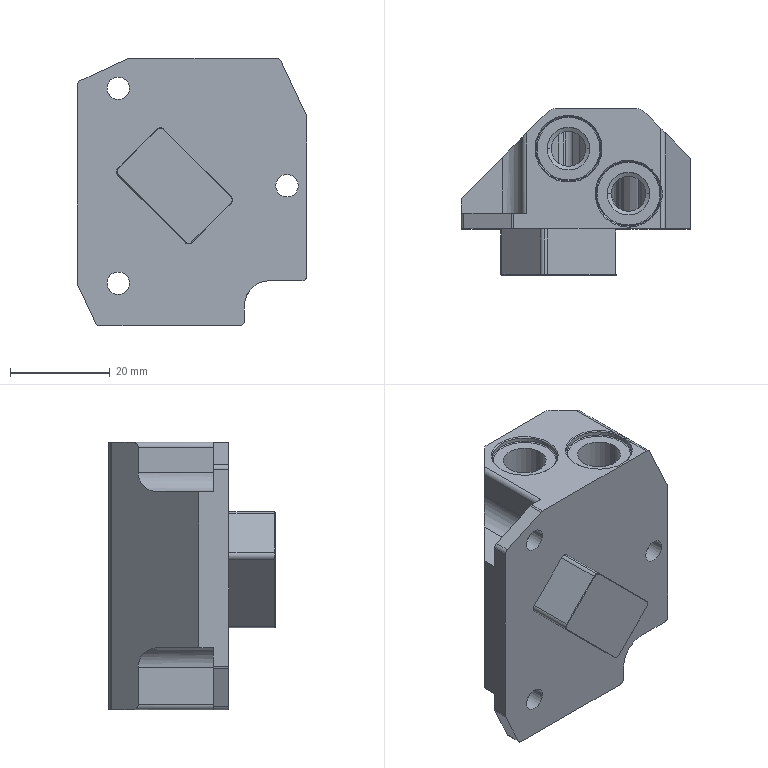NC program | NX | posted with a generic post | part box 46 x 33.25 x 53.5 mm
Lines 19 to 841 of 9227:
(动态粗 , TOOL : D10-30-D10-75-3T-ROUGH)
N36 T02 M6
N38 G53
N40 G17 G0 G90 X35.793 Y-2.826 B0. C0. S5500 M3
N42 G43 Z30.2 H2
N44 Z-24.5
N46 G94 G1 X35.768 Y-2.825 Z-24.656 F1500.
N48 X35.743 Y-2.824 Z-24.718
N50 X35.718 Y-2.823 Z-24.763
N52 X35.693 Y-2.822 Z-24.8
N54 X35.668 Y-2.821 Z-24.831
N56 X35.643 Y-2.82 Z-24.857
N58 X35.618 Y-2.819 Z-24.88
N60 X35.593 Y-2.818 Z-24.9
N62 X35.568 Y-2.817 Z-24.918
N64 X35.543 Y-2.816 Z-24.933
N66 X35.518 Y-2.815 Z-24.947
N68 X35.493 Y-2.814 Z-24.958
N70 X35.468 Y-2.813 Z-24.968
N72 X35.443 Y-2.812 Z-24.977
N74 X35.418 Y-2.811 Z-24.984
N76 X35.393 Y-2.81 Z-24.99
N78 X35.368 Y-2.809 Z-24.994
N80 X35.343 Y-2.808 Z-24.997
N82 X35.318 Y-2.807 Z-24.999
N84 X35.293 Y-2.806 Z-25.
N86 X33.787 Y-2.747
N88 G3 X32.775 Y-3.481 R1.01
N90 X32.348 Y-6.702 R13.384
N92 G1 X32.245 Y-11.061
N94 G2 X31.896 Y-13.227 R14.737
N96 X31.329 Y-15.21 R7.148
N98 X27.785 Y-23.176 R150.474
N100 X26.718 Y-25.28 R15.121
N102 X22.414 Y-28.199 R7.784
N104 X17.525 Y-28.893 R20.84
N106 X6.201 Y-28.999 R306.779
N108 G1 X-16.874 Y-28.998
N110 G2 X-21.685 Y-27.937 R14.794
N112 X-28.661 Y-24.862 R88.391
N114 X-31.659 Y-21.135 R7.243
N116 X-32.586 Y-16.368 R16.374
N118 X-32.747 Y-7.596 R145.919
N120 G1 X-32.75 Y-3.096
N122 G2 X-32.733 Y10.261 R991.956
N124 X-30.343 Y14.303 R5.749
N126 X-26.662 Y15.925 R9.882
N128 G3 X-24.702 Y16.523 R9.347
N130 X-24.139 Y17.376 R1.119
N132 X-23.808 Y21.173 R21.778
N134 G2 X-23.699 Y23.253 R13.999
N136 X-20.868 Y27.145 R6.06
N138 X-16.339 Y28.654 R11.322
N140 X-10.239 Y28.977 R49.941
N142 G1 X-1.314 Y29.
N144 X13.211 Y28.998
N146 G2 X17.775 Y28.028 R14.405
N148 X24.908 Y24.933 R98.139
N150 X28.234 Y23.354 R61.251
N152 X30.841 Y20.415 R7.126
N154 G1 X30.98 Y20.237
N156 X31.512 Y19.195
N158 G2 X32.063 Y16.21 R10.538
N160 X32.246 Y7.889 R121.537
N162 G1 X32.25 Y2.714
N164 G2 X32.234 Y-9.235 R902.524
N166 G3 X31.95 Y-10.575 R62.037
N168 G2 X31.884 Y-13.384 R26.459
N170 X31.369 Y-15.105 R6.543
N172 G1 X26.932 Y-24.621
N174 X26.338 Y-25.631
N176 X25.567 Y-26.511
N178 X24.643 Y-27.23
N180 X23.601 Y-27.762
N182 X22.477 Y-28.09
N184 G2 X16.086 Y-28.423 R88.323
N186 X3.336 Y-28.499 R660.995
N188 G1 X-15.051 Y-28.498
N190 G2 X-18.406 Y-28.176 R18.904
N192 X-20.71 Y-27.663 R7.341
N194 X-26.906 Y-25.084 R50.581
N196 X-28.468 Y-23.983 R10.692
N198 G1 X-29.381 Y-23.446
N200 X-30.261 Y-22.674
N202 X-30.98 Y-21.751
N204 X-31.512 Y-20.709
N206 X-31.84 Y-19.585
N208 G2 X-32.225 Y-10.708 R96.838
N210 G1 X-32.249 Y-1.108
N212 G2 X-32.232 Y8.223 R534.374
N214 X-31.934 Y9.881 R9.532
N216 X-26.362 Y15.669 R6.203
N218 G3 X-24.57 Y16.389 R3.889
N220 X-23.862 Y17.732 R2.705
N222 X-23.399 Y20.922 R18.234
N224 G2 X-22.838 Y23.021 R9.161
N226 G1 X-22.762 Y23.515
N228 X-22.37 Y24.619
N230 X-21.777 Y25.629
N232 X-21.005 Y26.509
N234 X-20.081 Y27.229
N236 X-19.039 Y27.762
N238 X-17.914 Y28.09
N240 G2 X-8.605 Y28.478 R100.527
N242 G1 X-0.355 Y28.499
N244 G2 X12.086 Y28.483 R926.244
N246 X14.656 Y28.2 R21.713
N248 X17.449 Y27.619 R6.654
N250 X26.375 Y23.663 R119.47
N252 X27.507 Y22.929 R30.959
N254 X29.381 Y21.933 R12.327
N256 G1 X30.261 Y21.161
N258 X30.86 Y20.391
N260 X30.261 Y21.161
N262 X29.381 Y21.933
N264 G3 X27.507 Y22.929 R12.327
N266 G1 X17.449 Y27.619
N268 G3 X14.656 Y28.2 R6.624
N270 G1 X-16.749
N272 X-17.914 Y28.09
N274 X-19.039 Y27.762
N276 X-20.081 Y27.229
N278 X-21.005 Y26.509
N280 X-21.777 Y25.629
N282 X-22.37 Y24.619
N284 X-22.762 Y23.515
N286 G3 X-23.224 Y19.783 R77.333
N288 G2 X-23.913 Y17.107 R8.828
N290 X-25.837 Y15.697 R2.696
N292 G3 X-26.589 Y15.628 R10.459
N294 G2 X-25.425 Y15.727 R25.281
N296 G3 X-23.638 Y17.249 R2.66
N298 X-22.95 Y19.454 R8.395
N300 G1 X-22.94 Y22.357
N302 G2 X-22.972 Y18.942 R91.453
N304 X-24.268 Y16.215 R4.314
N306 X-25.661 Y15.697 R1.792
N308 G3 X-23.723 Y16.556 R2.139
N310 X-22.95 Y18.084 R3.195
N312 G1 Y19.247
N314 G2 X-22.971 Y17.827 R14.78
N316 X-24.704 Y15.732 R2.841
N318 X-25.143 Y15.699 R6.429
N320 G3 X-23.597 Y16.317 R1.818
N322 X-22.95 Y17.469 R1.983
N324 G1 Y18.032
N326 G2 X-22.983 Y17.179 R3.888
N328 X-24.412 Y15.717 R2.152
N330 G1 X-24.786 Y15.7
N332 G3 X-23.244 Y16.394 R1.668
N334 X-22.95 Y17.418 R1.288
N336 G2 X-23.709 Y15.879 R1.538
N338 X-24.426 Y15.7 R1.168
N340 G3 X-22.95 Y17.059 R1.284
N342 G2 X-24.162 Y15.7 R1.183
N344 G3 X-22.959 Y16.708 R1.089
N346 G2 X-23.845 Y15.72 R1.054
N348 X-26.143 Y15.688 R53.417
N350 G3 X-31.95 Y9.5 R6.211
N352 G1 Y-18.42
N354 X-31.84 Y-19.585
N356 X-31.512 Y-20.709
N358 X-30.98 Y-21.751
N360 X-30.261 Y-22.674
N362 X-29.381 Y-23.446
N364 G3 X-26.506 Y-24.94 R24.613
N366 X-23.307 Y-26.404 R59.619
N368 G1 X-20.695 Y-27.619
N370 X-19.854 Y-27.939
N372 X-20.695 Y-27.619
N374 X-28.234 Y-24.103
N376 X-20.695 Y-27.619
N378 G3 X-18.075 Y-28.2 R6.608
N380 G1 X21.312
N382 G2 X21.972 Y-28.448 R1.005
N384 G1 X22.508 Y-28.919
N386 X23.998 Y-30.226 Z-24.9
N388 G3 X25.175 Y-30.43 R1.026 F15000.
N390 G1 X25.866 Y-30.088
N392 X26.549 Y-29.732
N394 G3 X28.082 Y-28.293 R4.702
N396 X30.353 Y-24.623 R45.308
N398 X32.163 Y-21.176 R57.483
N400 X33.537 Y-17.922 R42.581
N402 G1 X35.104 Y-13.729
N404 G3 X34.6 Y-12.477 R1.
N406 G1 X34.441 Y-12.401
N408 X32.654 Y-11.542 Z-25. F1500.
N410 G2 X32.103 Y-11.107 R1.163
N412 X31.95 Y-10.575 R1.013
N414 G1 Y16.907
N416 X31.84 Y18.071
N418 G2 X32.444 Y19.093 R1.01
N420 G1 X33.935 Y19.738
N422 X33.958 Y19.748 Z-24.999
N424 X33.981 Y19.758 Z-24.997
N426 X34.004 Y19.768 Z-24.994
N428 X34.027 Y19.778 Z-24.99
N430 X34.05 Y19.788 Z-24.984
N432 X34.073 Y19.797 Z-24.977
N434 X34.096 Y19.807 Z-24.968
N436 X34.119 Y19.817 Z-24.958
N438 X34.142 Y19.827 Z-24.947
N440 X34.165 Y19.837 Z-24.933
N442 X34.187 Y19.847 Z-24.918
N444 X34.21 Y19.857 Z-24.9
N446 X34.233 Y19.867 Z-24.88
N448 X34.256 Y19.877 Z-24.857
N450 X34.279 Y19.887 Z-24.831
N452 X34.302 Y19.897 Z-24.8
N454 X34.325 Y19.907 Z-24.763
N456 X34.348 Y19.917 Z-24.718
N458 X34.371 Y19.926 Z-24.656
N460 X34.394 Y19.936 Z-24.5
N462 G0 Z30.2
N464 X34.919 Y-8.983
N466 Z-20.25
N468 G1 X34.894 Y-8.988 Z-20.406
N470 X34.87 Y-8.992 Z-20.468
N472 X34.845 Y-8.997 Z-20.513
N474 X34.821 Y-9.002 Z-20.55
N476 X34.796 Y-9.007 Z-20.581
N478 X34.772 Y-9.011 Z-20.607
N480 X34.747 Y-9.016 Z-20.63
N482 X34.723 Y-9.021 Z-20.65
N484 X34.698 Y-9.025 Z-20.668
N486 X34.673 Y-9.03 Z-20.683
N488 X34.649 Y-9.035 Z-20.697
N490 X34.624 Y-9.039 Z-20.708
N492 X34.6 Y-9.044 Z-20.718
N494 X34.575 Y-9.049 Z-20.727
N496 X34.551 Y-9.053 Z-20.734
N498 X34.526 Y-9.058 Z-20.74
N500 X34.502 Y-9.063 Z-20.744
N502 X34.477 Y-9.067 Z-20.747
N504 X34.452 Y-9.072 Z-20.749
N506 X34.428 Y-9.077 Z-20.75
N508 X32.722 Y-9.402
N510 G3 X31.906 Y-10.295 R1.01
N512 G2 X31.056 Y-14.012 R14.1
N514 X28.401 Y-20.262 R75.825
N516 X26.858 Y-23.475 R47.618
N518 X22.769 Y-26.709 R7.485
N520 X19.592 Y-27.417 R16.665
N522 G3 X18.824 Y-27.805 R19.475
N524 G1 X17.849 Y-28.1
N526 X17.214 Y-28.163
N528 G3 X19.551 Y-27.417 R4.892
N530 X22.182 Y-26.533 R101.684
N532 X26.36 Y-23.095 R8.995
N534 X28.937 Y-18.301 R32.428
N536 X30.941 Y-13.227 R41.328
N538 G1 X31.477 Y-12.224
N540 X31.83 Y-11.061
N542 X31.477 Y-12.224
N544 G2 X30.373 Y-14.168 R37.231
N546 G3 X27.811 Y-19.458 R525.404
N548 G2 X25.412 Y-23.188 R16.8
N550 X21.65 Y-25.856 R11.889
N552 G3 X20.769 Y-26.364 R2.983
N554 G2 X19.492 Y-27.448 R4.465
N556 G3 X20.841 Y-26.277 R4.557
N558 G2 X22.786 Y-24.915 R28.771
N560 G3 X26.923 Y-20.257 R14.47
N562 X29.554 Y-15.145 R84.07
N564 G2 X30.065 Y-14.292 R3.495
N566 X30.981 Y-14.073 R1.001
N568 X31.604 Y-14.549 Z-20.709 R1.062
N570 G1 X32.278 Y-15.516 Z-20.65
N572 X32.544 Y-15.905 F15000.
N574 X32.826 Y-16.283
N576 G3 X33.928 Y-16.522 R1.001
N578 X34.616 Y-15.84 R1.056
N580 X34.28 Y-14.769 R1.001
N582 G1 X33.347 Y-14.028
N584 X32.783 Y-13.576 Z-20.686 F1500.
N586 X32.212 Y-13.133 Z-20.723
N588 G3 X31.711 Y-12.961 Z-20.75 R1.005
N590 X30.88 Y-13.325 R1.002
N592 G2 X29.706 Y-14.636 R9.525
N594 G3 X28.14 Y-17.08 R16.696
N596 G2 X25.541 Y-21.266 R33.612
N598 X22.103 Y-24.604 R19.075
N600 G3 X21.565 Y-25.13 R2.381
N602 G2 X20.801 Y-26.325 R4.553
N604 G3 X21.565 Y-25.13 R4.553
N606 G2 X22.53 Y-24.018 R5.772
N608 G3 X27.3 Y-17.885 R25.805
N610 G2 X29.059 Y-15.12 R26.394
N612 G1 X29.17 Y-15.02
N614 G2 X30.131 Y-14.984 R1.001
N616 G1 X30.842 Y-15.439 Z-20.707
N618 X31.544 Y-15.906 Z-20.665
N620 X31.79 Y-16.068 Z-20.65
N622 X32.153 Y-16.303 F15000.
N624 X32.506 Y-16.552
N626 G2 X32.324 Y-18.173 R1.
N628 X31.88 Y-18.368 R1.466
N630 X30.801 Y-16.905 R1.
N632 G1 X31.481 Y-15.568 Z-20.726 F1500.
N634 G3 X31.561 Y-15.098 Z-20.75 R1.011
N636 X29.93 Y-14.401 R1.
N638 G1 X28.753 Y-15.336
N640 G3 X26.942 Y-17.681 R15.325
N642 G2 X22.471 Y-23.318 R39.283
N644 G3 X21.916 Y-24.078 R2.888
N646 G1 X21.604 Y-25.057
N648 X22.005 Y-23.847
N650 G2 X23.28 Y-22.075 R12.371
N652 G3 X27.053 Y-17.004 R85.206
N654 G2 X28.422 Y-15.421 R8.427
N656 G1 X29.115 Y-15.048
N658 G3 X27.629 Y-15.978 R6.454
N660 X25.208 Y-18.817 R24.169
N662 X22.369 Y-22.517 R82.134
N664 X22.008 Y-23.275 R2.038
N666 G1 X21.935 Y-24.016
N668 G2 X22.063 Y-22.987 R6.701
N670 X23.285 Y-20.905 R9.096
N672 X26.806 Y-16.471 R46.103
N674 X27.781 Y-15.682 R3.267
N676 G3 X28.254 Y-15.508 R2.699
N678 G2 X27.496 Y-15.78 R5.801
N680 G3 X25.578 Y-17.364 R7.119
N682 X22.344 Y-21.603 R25.212
N684 X22.036 Y-22.416 R1.987
N686 G1 X22.017 Y-23.187
N688 X22.038 Y-22.266
N690 G2 X22.97 Y-20.275 R5.838
N692 X26.279 Y-16.384 R18.594
N694 X26.95 Y-15.934 R3.562
N696 G1 X27.604 Y-15.735
N698 G3 X26.331 Y-16.183 R6.188
N700 X23.778 Y-18.524 R10.161
N702 X22.073 Y-21.226 R10.194
N704 X22.036 Y-22.347 R5.834
N706 G2 X22.058 Y-21.191 R10.596
N708 X23.243 Y-18.888 R6.735
N710 X26.005 Y-16.189 R9.856
N712 X26.958 Y-15.931 R1.713
N714 G3 X24.867 Y-16.739 R3.341
N716 X22.075 Y-20.277 R8.813
N718 X22.036 Y-21.409 R5.651
N720 G2 X22.058 Y-20.252 R10.443
N722 X23.441 Y-17.828 R6.024
N724 X25.691 Y-16.076 R6.255
N726 G1 X26.359 Y-15.99
N728 G3 X24.011 Y-16.909 R3.554
N730 X22.071 Y-19.442 R6.352
N732 X22.036 Y-20.451 R4.327
N734 G2 X22.089 Y-19.278 R4.722
N736 X25.128 Y-16.088 R5.398
N738 X25.749 Y-16.05 R2.961
N740 G3 X23.655 Y-16.728 R2.866
N742 X22.068 Y-18.726 R4.655
N744 X22.036 Y-19.618 R4.413
N746 G2 X22.065 Y-18.652 R5.206
N748 X24.653 Y-16.066 R4.087
N750 G1 X25.201 Y-16.05
N752 G3 X23.023 Y-16.825 R2.747
N754 X22.058 Y-18.173 R2.99
N756 X22.036 Y-18.9 R12.294
N758 G2 X22.068 Y-18.046 R3.962
N760 X24.165 Y-16.059 R3.109
N762 G1 X24.631 Y-16.05
N764 G3 X22.582 Y-16.859 R2.389
N766 X22.036 Y-18.268 R1.614
N768 G2 X22.192 Y-17.273 R1.791
N770 X23.708 Y-16.059 R2.402
N772 G1 X24.1 Y-16.05
N774 G3 X22.066 Y-17.296 R1.929
N776 X22.036 Y-17.831 R4.435
N778 G2 X22.719 Y-16.35 R1.512
N780 X23.672 Y-16.05 R1.32
N782 G3 X22.073 Y-16.998 R1.488
N784 X22.036 Y-17.482 R3.147
N786 G2 X23.309 Y-16.05 R1.25
N788 G3 X22.494 Y-16.246 R1.346
N790 X22.041 Y-17.096 R1.076
N792 G1 X22.036 Y-17.188
N794 G2 X22.221 Y-16.519 R1.243
N796 X22.754 Y-16.119 R1.034
N798 X23.993 Y-16.724 R1.01
N800 G1 X24.682 Y-18.528
N802 X24.69 Y-18.551 Z-20.749
N804 X24.699 Y-18.575 Z-20.747
N806 X24.708 Y-18.598 Z-20.744
N808 X24.717 Y-18.621 Z-20.74
N810 X24.726 Y-18.645 Z-20.734
N812 X24.735 Y-18.668 Z-20.727
N814 X24.744 Y-18.692 Z-20.718
N816 X24.753 Y-18.715 Z-20.708
N818 X24.762 Y-18.738 Z-20.697
N820 X24.771 Y-18.762 Z-20.683
N822 X24.78 Y-18.785 Z-20.668
N824 X24.789 Y-18.808 Z-20.65
N826 X24.798 Y-18.832 Z-20.63
N828 X24.806 Y-18.855 Z-20.607
N830 X24.815 Y-18.878 Z-20.581
N832 X24.824 Y-18.902 Z-20.55
N834 X24.833 Y-18.925 Z-20.513
N836 X24.842 Y-18.948 Z-20.468
N838 X24.851 Y-18.972 Z-20.406
N840 X24.86 Y-18.995 Z-20.25
N842 G0 Z30.2
N844 X-13.457 Y-31.172
N846 Z-20.25
N848 G1 X-13.461 Y-31.148 Z-20.406
N850 X-13.464 Y-31.123 Z-20.468
N852 X-13.468 Y-31.098 Z-20.513
N854 X-13.472 Y-31.073 Z-20.55
N856 X-13.475 Y-31.049 Z-20.581
N858 X-13.479 Y-31.024 Z-20.607
N860 X-13.483 Y-30.999 Z-20.63
N862 X-13.486 Y-30.975 Z-20.65
N864 X-13.49 Y-30.95 Z-20.668
N866 X-13.494 Y-30.925 Z-20.683
N868 X-13.498 Y-30.9 Z-20.697
N870 X-13.501 Y-30.876 Z-20.708
N872 X-13.505 Y-30.851 Z-20.718
N874 X-13.509 Y-30.826 Z-20.727
N876 X-13.512 Y-30.801 Z-20.734
N878 X-13.516 Y-30.777 Z-20.74
N880 X-13.52 Y-30.752 Z-20.744
N882 X-13.523 Y-30.727 Z-20.747
N884 X-13.527 Y-30.703 Z-20.749
N886 X-13.531 Y-30.678 Z-20.75
N888 X-13.778 Y-29.022
N890 G3 X-14.677 Y-28.166 R1.01
N892 G2 X-16.399 Y-27.916 R20.903
N894 X-21.244 Y-26.649 R17.69
N896 X-27.074 Y-24.047 R73.374
N898 X-30.423 Y-19.963 R7.43
N900 X-31.291 Y-15.297 R16.875
N902 G1 X-31.418 Y-12.413
N904 X-31.472 Y-12.234
N906 G3 X-32.02 Y-11.763 R1.004
N908 G1 X-32.461 Y-11.608
N910 X-34.33 Y-10.947 Z-20.65
N912 X-34.597 Y-10.851 F15000.
N914 X-34.868 Y-10.769
N916 G3 X-35.932 Y-12.234 R1.
N918 G1 X-35.815 Y-12.446
N920 X-35.689 Y-12.653
N922 G3 X-33.994 Y-12.489 R1.
N924 X-33.893 Y-11.949 Z-20.678 R1.135 F1500.
N926 G1 X-33.9 Y-10.522 Z-20.75
N928 G2 X-33.515 Y-9.61 R1.057
N930 X-31.906 Y-10.301 R1.
N932 G1 X-31.831 Y-11.058
N934 G2 X-31.325 Y-12.732 R28.885
N936 X-30.854 Y-16.508 R148.155
N938 G3 X-29.566 Y-20.596 R11.254
N940 X-26.196 Y-23.864 R9.827
N942 X-18.743 Y-27.088 R29.083
N944 G2 X-16.891 Y-27.505 R64.827
N946 G1 X-16.327 Y-27.803
N948 X-15.351 Y-28.1
N950 G2 X-17.226 Y-27.323 R6.073
N952 G3 X-21.161 Y-25.747 R202.118
N954 G2 X-25.892 Y-23.291 R24.946
N956 X-29.663 Y-17.993 R10.083
N958 X-30.581 Y-14. R33.2
N960 G3 X-30.906 Y-13.293 R1.294
N962 G1 X-31.471 Y-12.235
N964 X-30.906 Y-13.293
N966 G2 X-30.391 Y-14.328 R2.424
N968 G3 X-29.314 Y-17.877 R53.28
N970 X-24.691 Y-23.496 R11.223
N972 X-19.336 Y-26.124 R30.901
N974 G2 X-17.933 Y-26.742 R11.178
N976 G1 X-17.226 Y-27.323
N978 G3 X-20.119 Y-25.393 R11.781
N980 G2 X-24.276 Y-23.032 R33.212
N982 X-28.755 Y-17.218 R12.639
N984 G3 X-29.787 Y-14.594 R84.708
N986 G1 X-29.976 Y-14.363
N988 G3 X-30.845 Y-14.166 R1.002
N990 X-31.338 Y-14.446 Z-20.721 R1.101
N992 G1 X-32.398 Y-15.373 Z-20.65
N994 X-33.638 Y-16.457 F15000.
N996 G2 X-34.511 Y-16.73 R1.128
N998 X-34.865 Y-14.873 R1.
N1000 G1 X-33.357 Y-14.007
N1002 X-32.661 Y-13.604 Z-20.691 F1500.
N1004 X-31.96 Y-13.211 Z-20.731
N1006 X-31.785 Y-13.146 Z-20.741
N1008 X-31.602 Y-13.113 Z-20.75
N1010 G2 X-30.756 Y-13.476 R1.001
N1012 G1 X-30.135 Y-14.233
N1014 G2 X-29.419 Y-15.161 R2.282
N1016 G3 X-27.79 Y-18.449 R67.036
N1018 X-22.717 Y-23.541 R14.296
N1020 X-19.074 Y-25.645 R422.71
N1022 G2 X-18.535 Y-26.039 R5.066
N1024 G1 X-18.013 Y-26.676
N1026 G3 X-20.333 Y-24.527 R8.106
N1028 G2 X-24.016 Y-21.888 R35.914
N1030 X-27.715 Y-17.185 R16.834
N1032 G3 X-28.869 Y-15.239 R17.423
N1034 G1 X-29.071 Y-15.072
N1036 G3 X-30.052 Y-15.051 R1.001
N1038 G1 X-31.705 Y-16.145 Z-20.65
N1040 X-32.054 Y-16.374 F15000.
N1042 X-32.393 Y-16.616
N1044 G3 X-32.162 Y-18.262 R1.007
N1046 X-30.783 Y-16.92 R1.
N1048 G1 X-31.48 Y-15.574 Z-20.727 F1500.
N1050 G2 X-31.565 Y-15.12 Z-20.75 R1.013
N1052 X-29.932 Y-14.399 R1.
N1054 G3 X-28.851 Y-15.225 R10.073
N1056 G2 X-27.639 Y-16.861 R10.451
N1058 G3 X-23.913 Y-21.428 R20.905
N1060 X-20.195 Y-24.259 R45.953
N1062 G2 X-18.96 Y-25.331 R6.532
N1064 G1 X-18.66 Y-25.888
N1066 G3 X-20.266 Y-23.841 R5.548
N1068 G2 X-23.617 Y-20.924 R71.502
N1070 X-27.046 Y-16.757 R31.261
N1072 G3 X-28.004 Y-15.642 R5.431
N1074 G1 X-28.101 Y-15.585
N1076 G3 X-29.067 Y-15.758 R1.001
N1078 G1 X-30.547 Y-17.076 Z-20.65
N1080 X-31.303 Y-17.749 F15000.
N1082 G3 X-30.331 Y-19.448 R1.
N1084 X-29.716 Y-19.08 R1.161
N1086 X-29.599 Y-17.997 R1.001
N1088 G1 X-29.864 Y-17.473
N1090 X-30.42 Y-16.364 Z-20.713 F1500.
N1092 G2 X-30.445 Y-15.64 Z-20.75 R1.001
N1094 X-29.03 Y-15.093 R1.
N1096 X-27.781 Y-15.781 R12.344
N1098 X-26.211 Y-17.491 R13.038
N1100 G3 X-20.943 Y-22.853 R36.83
N1102 G2 X-19.303 Y-24.527 R10.316
N1104 G3 X-19.034 Y-25.187 R6.262
N1106 G2 X-19.332 Y-24.395 R4.429
N1108 G3 X-20.867 Y-22.456 R8.134
N1110 G2 X-26.06 Y-16.897 R88.533
N1112 G3 X-27.204 Y-15.865 R5.049
N1114 G1 X-28.124 Y-15.577
N1116 G2 X-27.048 Y-15.926 R14.317
N1118 X-25.149 Y-17.582 R9.073
N1120 G3 X-20.541 Y-22.401 R793.67
N1122 G2 X-19.49 Y-23.804 R6.457
N1124 G1 X-19.446 Y-23.948
N1126 G2 X-20.931 Y-24.994 R1.
N1128 X-21.356 Y-24.518 Z-20.717 R1.087
N1130 G1 X-21.987 Y-23.343 Z-20.65
N1132 G3 X-22.367 Y-22.856 R1.216 F15000.
N1134 X-23.906 Y-23.948 R1.
N1136 G1 X-23.808 Y-24.299
N1138 X-23.694 Y-24.646
N1140 G3 X-23.003 Y-25.204 R1.002
N1142 G1 X-21.595 Y-25.517
N1144 X-20.394 Y-25.779 Z-20.712 F1500.
N1146 G3 X-19.677 Y-25.616 Z-20.75 R1.001
N1148 X-19.287 Y-24.502 R1.
N1150 G1 X-19.546 Y-23.539
N1152 G3 X-21.065 Y-21.322 R8.951
N1154 X-25.29 Y-16.814 R65.506
N1156 X-26.398 Y-16.01 R3.98
N1158 G1 X-26.961 Y-15.93
N1160 X-27.212 Y-15.854
N1162 G3 X-26.425 Y-15.986 R2.968
N1164 G2 X-24.823 Y-17.012 R4.73
N1166 X-20.233 Y-21.97 R37.038
N1168 X-19.506 Y-23.315 R4.238
N1170 G1 X-19.447 Y-23.901
N1172 G3 X-20.251 Y-21.506 R4.202
N1174 X-24.76 Y-16.574 R22.329
N1176 X-25.751 Y-16.05 R2.362
N1178 G1 X-26.534 Y-15.973
N1180 G2 X-25.49 Y-16.093 R10.153
N1182 X-23.546 Y-17.359 R6.184
N1184 X-20.002 Y-21.511 R18.502
N1186 X-19.536 Y-22.653 R3.145
N1188 G1 X-19.521 Y-23.149
N1190 G3 X-19.59 Y-22.127 R6.741
N1192 X-20.941 Y-19.605 R7.555
N1194 X-24.181 Y-16.427 R13.415
N1196 X-25.074 Y-16.05 R2.04
N1198 G1 X-25.749
N1200 G2 X-24.68 Y-16.111 R3.709
N1202 X-22.471 Y-17.574 R6.507
N1204 X-19.734 Y-21.215 R11.626
N1206 X-19.536 Y-22.477 R2.427
N1208 G3 X-19.674 Y-20.986 R4.296
N1210 X-21.881 Y-17.662 R9.08
N1212 X-24.082 Y-16.085 R6.581
N1214 X-25.016 Y-16.05 R4.105
N1216 G2 X-24.01 Y-16.08 R5.105
N1218 X-21.903 Y-17.396 R5.411
N1220 X-19.573 Y-20.805 R8.403
N1222 X-19.536 Y-21.664 R3.636
N1224 G3 X-19.636 Y-20.256 R4.763
N1226 X-23.197 Y-16.129 R7.312
N1228 G1 X-23.549 Y-16.05
N1230 X-24.262
N1232 G2 X-23.256 Y-16.08 R5.107
N1234 X-21.134 Y-17.492 R5.002
N1236 X-19.545 Y-20.105 R6.146
N1238 G1 X-19.536 Y-20.806
N1240 G3 X-19.644 Y-19.423 R4.383
N1242 X-22.55 Y-16.109 R5.744
N1244 X-23.481 Y-16.05 R3.142
N1246 G2 X-22.443 Y-16.115 R3.432
N1248 X-20.068 Y-18.172 R4.947
N1250 X-19.536 Y-19.444 R3.169
N1252 G1 Y-20.006
N1254 G3 X-19.652 Y-18.672 R3.869
N1256 X-21.963 Y-16.097 R4.46
N1258 X-22.783 Y-16.05 R2.828
N1260 G2 X-21.79 Y-16.127 R2.762
N1262 X-19.542 Y-18.696 R3.913
N1264 G1 X-19.536 Y-19.221
N1266 G3 X-20.412 Y-16.833 R2.935
N1268 X-21.566 Y-16.064 R2.389
N1270 G1 X-22.176 Y-16.05
N1272 G2 X-21.255 Y-16.133 R2.354
N1274 X-19.543 Y-18.131 R3.013
N1276 G1 X-19.536 Y-18.618
N1278 G3 X-21.033 Y-16.086 R2.451
N1280 X-21.63 Y-16.05 R3.144
N1282 G2 X-20.109 Y-16.652 R1.681
N1284 X-19.536 Y-17.752 R1.919
N1286 G1 Y-18.052
N1288 G3 X-20.662 Y-16.096 R1.879
N1290 X-21.183 Y-16.05 R2.304
N1292 G2 X-19.854 Y-16.654 R1.392
N1294 X-19.536 Y-17.616 R1.308
N1296 G3 X-20.444 Y-16.087 R1.412
N1298 X-20.891 Y-16.05 R3.683
N1300 G2 X-19.536 Y-17.26 R1.192
N1302 G3 X-20.545 Y-16.059 R1.088
N1304 X-21.605 Y-16.752 R1.01
N1306 G1 X-22.182 Y-18.528
N1308 X-22.19 Y-18.552 Z-20.749
N1310 X-22.198 Y-18.575 Z-20.747
N1312 X-22.205 Y-18.599 Z-20.744
N1314 X-22.213 Y-18.623 Z-20.74
N1316 X-22.221 Y-18.647 Z-20.734
N1318 X-22.229 Y-18.671 Z-20.727
N1320 X-22.236 Y-18.694 Z-20.718
N1322 X-22.244 Y-18.718 Z-20.708
N1324 X-22.252 Y-18.742 Z-20.697
N1326 X-22.259 Y-18.766 Z-20.683
N1328 X-22.267 Y-18.789 Z-20.668
N1330 X-22.275 Y-18.813 Z-20.65
N1332 X-22.283 Y-18.837 Z-20.63
N1334 X-22.29 Y-18.861 Z-20.607
N1336 X-22.298 Y-18.885 Z-20.581
N1338 X-22.306 Y-18.908 Z-20.55
N1340 X-22.313 Y-18.932 Z-20.513
N1342 X-22.321 Y-18.956 Z-20.468
N1344 X-22.329 Y-18.98 Z-20.406
N1346 X-22.337 Y-19.003 Z-20.25
N1348 G0 Z30.2
N1350 X-4.094 Y31.178
N1352 Z-19.5
N1354 G1 Y31.153 Z-19.656
N1356 Y31.128 Z-19.718
N1358 Y31.103 Z-19.763
N1360 Y31.078 Z-19.8
N1362 Y31.053 Z-19.831
N1364 Y31.028 Z-19.857
N1366 Y31.003 Z-19.88
N1368 Y30.978 Z-19.9
N1370 Y30.953 Z-19.918
N1372 Y30.928 Z-19.933
N1374 Y30.903 Z-19.947
N1376 Y30.878 Z-19.958
N1378 Y30.853 Z-19.968
N1380 X-4.093 Y30.828 Z-19.977
N1382 Y30.803 Z-19.984
N1384 Y30.778 Z-19.99
N1386 Y30.753 Z-19.994
N1388 Y30.728 Z-19.997
N1390 Y30.703 Z-19.999
N1392 Y30.678 Z-20.
N1394 X-4.09 Y29.158
N1396 G3 X-3.174 Y28.155 R1.01
N1398 G2 X-1.36 Y27.914 R31.351
N1400 G3 X3.739 Y27.732 R46.669
N1402 G1 X4.997 Y28.092
N1404 X5.707 Y28.158
N1406 X4.997 Y28.092
N1408 G2 X3.351 Y27.643 R15.286
N1410 X-1.126 Y27.663 R20.178
N1412 G1 X-1.267 Y27.712
N1414 G2 X-1.715 Y29.254 R1.1
N1416 X-0.69 Y29.794 Z-19.939 R1.133
N1418 G1 X0.074 Y29.805 Z-19.9
N1420 X2.473 Y29.839 F15000.
N1422 X3.449 Y29.848 Z-19.949 F1500.
N1424 G2 X4.295 Y29.373 Z-20. R1.099
N1426 X3.883 Y27.771 R1.1
N1428 X2.035 Y27.364 R5.085
N1430 X-0.653 Y27.417 R10.798
N1432 G1 X-1.381 Y27.77
N1434 X-2.494 Y28.091
N1436 X-1.381 Y27.77
N1438 G3 X0.072 Y27.173 R5.086
N1440 X2.639 Y27.146 R6.515
N1442 G1 X2.841 Y27.242
N1444 G3 X3.175 Y28.558 R1.1
N1446 X2.189 Y29.217 Z-19.937 R1.127
N1448 G1 X1.461 Y29.29 Z-19.9
N1450 X0.991 Y29.337 F15000.
N1452 X0.444 Y29.396 Z-19.928 F1500.
N1454 X-0.105 Y29.438 Z-19.956
N1456 G3 X-0.884 Y29.077 Z-20. R1.116
N1458 X-0.565 Y27.357 R1.1
N1460 X2.247 Y26.863 R4.2
N1462 X2.848 Y27.248 R2.033
N1464 G1 X3.752 Y27.704
N1466 X2.848 Y27.248
N1468 G2 X1.295 Y26.71 R1.945
N1470 X-0.046 Y27.015 R2.698
N1472 G1 X-0.346 Y27.246
N1474 G3 X1.931 Y26.609 R2.517
N1476 X2.481 Y26.965 R2.206
N1478 G2 X0.896 Y26.516 R1.681
N1480 X0.082 Y26.917 R1.451
N1482 G3 X1.549 Y26.387 R1.853
N1484 X2.146 Y26.708 R1.405
N1486 G2 X0.444 Y26.639 R1.239
N1488 G1 X0.591 Y26.532
N1490 X0.745 Y26.437
N1492 G3 X1.829 Y26.478 R1.039
N1494 X2.22 Y27.737 R1.01
N1496 G1 X1.524 Y29.341
N1498 X1.514 Y29.364 Z-19.999
N1500 X1.504 Y29.387 Z-19.997
N1502 X1.494 Y29.409 Z-19.994
N1504 X1.484 Y29.432 Z-19.99
N1506 X1.474 Y29.455 Z-19.984
N1508 X1.464 Y29.478 Z-19.977
N1510 X1.454 Y29.501 Z-19.968
N1512 X1.444 Y29.524 Z-19.958
N1514 X1.434 Y29.547 Z-19.947
N1516 X1.424 Y29.57 Z-19.933
N1518 X1.414 Y29.593 Z-19.918
N1520 X1.404 Y29.616 Z-19.9
N1522 X1.394 Y29.639 Z-19.88
N1524 X1.384 Y29.662 Z-19.857
N1526 X1.374 Y29.685 Z-19.831
N1528 X1.364 Y29.708 Z-19.8
N1530 X1.354 Y29.731 Z-19.763
N1532 X1.344 Y29.753 Z-19.718
N1534 X1.334 Y29.776 Z-19.656
N1536 X1.325 Y29.799 Z-19.5
N1538 G0 Z30.2
N1540 X25.008 Y-21.219
N1542 Z-16.5
N1544 G1 X24.984 Y-21.222 Z-16.656
N1546 X24.959 Y-21.226 Z-16.718
N1548 X24.934 Y-21.229 Z-16.763
N1550 X24.909 Y-21.233 Z-16.8
N1552 X24.885 Y-21.236 Z-16.831
N1554 X24.86 Y-21.24 Z-16.857
N1556 X24.835 Y-21.244 Z-16.88
N1558 X24.81 Y-21.247 Z-16.9
N1560 X24.786 Y-21.251 Z-16.918
N1562 X24.761 Y-21.254 Z-16.933
N1564 X24.736 Y-21.258 Z-16.947
N1566 X24.711 Y-21.261 Z-16.958
N1568 X24.687 Y-21.265 Z-16.968
N1570 X24.662 Y-21.269 Z-16.977
N1572 X24.637 Y-21.272 Z-16.984
N1574 X24.612 Y-21.276 Z-16.99
N1576 X24.588 Y-21.279 Z-16.994
N1578 X24.563 Y-21.283 Z-16.997
N1580 X24.538 Y-21.287 Z-16.999
N1582 X24.513 Y-21.29 Z-17.
N1584 X22.856 Y-21.53
N1586 G3 X21.995 Y-22.436 R1.01
N1588 G1 X21.941 Y-23.023
N1590 G2 X21.17 Y-24.913 R6.09
N1592 X19.735 Y-26.364 R6.09
N1594 X17.487 Y-27.231 R6.133
N1596 X11.809 Y-27.66 R35.814
N1598 X1.684 Y-27.7 R706.005
N1600 G1 X-12.392 Y-27.698
N1602 G2 X-14.432 Y-27.256 R5.98
N1604 X-16.336 Y-26.851 R6.062
N1606 X-18.026 Y-25.707 R6.09
N1608 X-19.15 Y-24.003 R6.09
N1610 G1 X-19.441 Y-23.02
N1612 X-19.496 Y-22.422
N1614 X-19.441 Y-23.02
N1616 G3 X-18.672 Y-24.91 R6.09
N1618 X-17.238 Y-26.362 R6.09
N1620 X-15.357 Y-27.155 R6.09
N1622 X-10.439 Y-27.385 R42.559
N1624 G1 X-3.839 Y-27.399
N1626 X11.92 Y-27.398
N1628 G2 X16.835 Y-27.262 R53.504
N1630 G1 X17.854 Y-27.156
N1632 X16.835 Y-27.262
N1634 X-14.336
N1636 G3 X-15.28 Y-27.912 R1.01
N1638 G1 X-15.913 Y-29.568
N1640 X-15.922 Y-29.591 Z-16.999
N1642 X-15.93 Y-29.614 Z-16.997
N1644 X-15.939 Y-29.638 Z-16.994
N1646 X-15.948 Y-29.661 Z-16.99
N1648 X-15.957 Y-29.684 Z-16.984
N1650 X-15.966 Y-29.708 Z-16.977
N1652 X-15.975 Y-29.731 Z-16.968
N1654 X-15.984 Y-29.754 Z-16.958
N1656 X-15.993 Y-29.778 Z-16.947
N1658 X-16.002 Y-29.801 Z-16.933
N1660 X-16.011 Y-29.825 Z-16.918
N1662 X-16.02 Y-29.848 Z-16.9
N1664 X-16.029 Y-29.871 Z-16.88
N1666 X-16.038 Y-29.895 Z-16.857
N1668 X-16.046 Y-29.918 Z-16.831
N1670 X-16.055 Y-29.941 Z-16.8
N1672 X-16.064 Y-29.965 Z-16.763
N1674 X-16.073 Y-29.988 Z-16.718